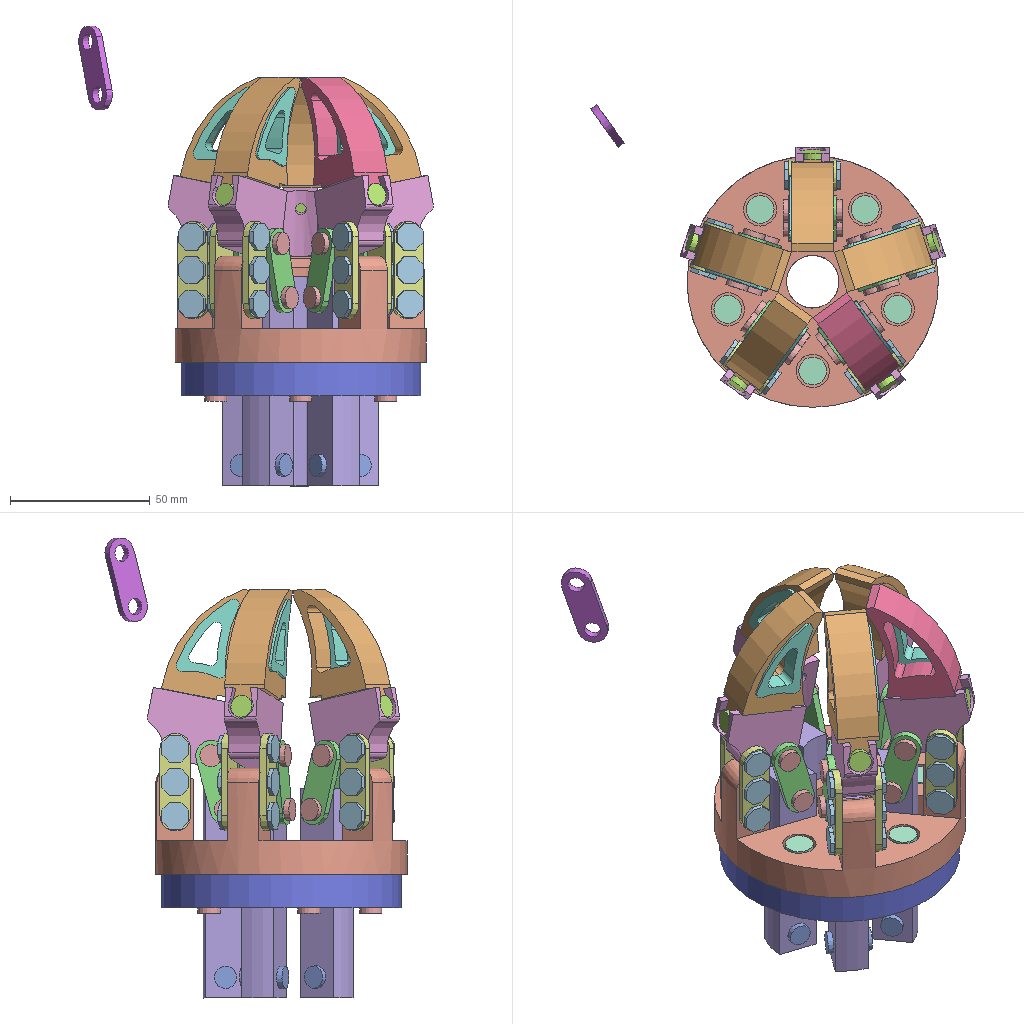Assembly | NX | 14 different items | 123 placed | box 127 x 108 x 165 mm
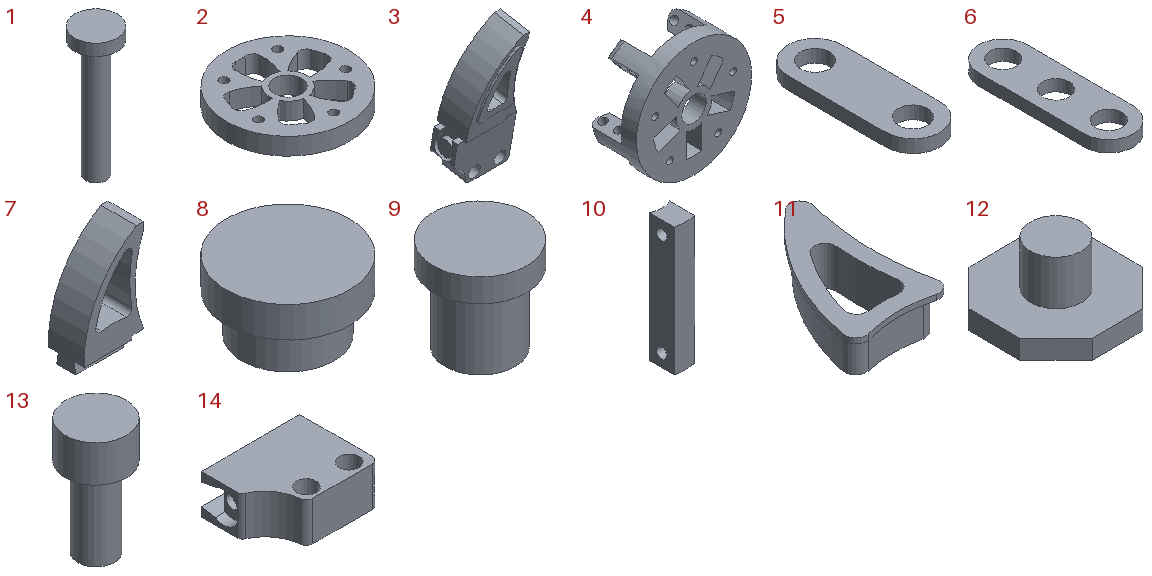Parts list (item | quantity | parent item | size | volume | features):
1 | x5 | in 3 | 8 x 8 x 24.4 mm | 389.557 mm3 | features DATUM_CSYS 2, EXTRUDE 2, SKETCH 1
2 | x1 | - | 86 x 86 x 12 mm | 44699 mm3 | features DATUM_CSYS 4, EXTRUDE 4, SKETCH 3
3 | x5 | - | - | 14028 mm3 | features DATUM_CSYS 17, EXTRUDE 15, SKETCH 13, CPROJ 4, BLEND 2
4 | x1 | - | 90 x 38 x 90 mm | 71655 mm3 | features DATUM_CSYS 9, SKETCH 8, EXTRUDE 7, CBORE_HOLE 5, CPROJ 1, HOLE PACKAGE 1, SWP104 1
5 | x11 | - | 11 x 31 x 2.6 mm | 672.06 mm3 | features DATUM_CSYS 2, EXTRUDE 1, SKETCH 1
6 | x10 | - | 11 x 35 x 2.6 mm | 712.946 mm3 | features DATUM_CSYS 2, EXTRUDE 1, SKETCH 1
7 | x5 | in 3 | - | 6914 mm3 | features DATUM_CSYS 4, EXTRUDE 3, SKETCH 3, CPROJ 2
8 | x25 | - | 8 x 8 x 4.5 mm | 171.217 mm3 | features CYLINDER 2, DATUM_CSYS 1
9 | x10 | - | 8 x 8 x 8 mm | 270.177 mm3 | features CYLINDER 2, DATUM_CSYS 1
10 | x5 | - | 12 x 15.351 x 75 mm | 12124 mm3 | features DATUM_CSYS 3, EXTRUDE 2, SKETCH 2
11 | x5 | in 3 | 18.409 x 28.891 x 7.4 mm | 1102 mm3 | features DATUM_CSYS 4, EXTRUDE 3, SKETCH 3, BLEND 1, CPROJ 1
12 | x30 | - | 9.657 x 9.657 x 5 mm | 159.865 mm3 | features DATUM_CSYS 2, EXTRUDE 2, SKETCH 1
13 | x5 | - | 10 x 10 x 19 mm | 838.805 mm3 | features DATUM_CSYS 2, EXTRUDE 2, SKETCH 1
14 | x5 | in 3 | 30 x 24 x 12 mm | 5622 mm3 | features DATUM_CSYS 7, EXTRUDE 7, SKETCH 6, BLEND 1, CPROJ 1
Mates (type | each side: item.copy, entity, surface, feature):
In the top assembly
Fix | assembly component | 6 times
Bond | 12.1 component | assembly component | 34 times
Bond | assembly component | 20 times
LinearPattern | assembly axis | assembly csys | assembly csys | assembly csys | 2 times
Bond | 6.1 component | assembly component | 10 times
CircularPattern | assembly axis | assembly csys | assembly csys | assembly csys | assembly csys | assembly csys | 16 times
Bond | 5.1 component | assembly component | 15 times
LinearPattern | assembly axis | assembly csys | assembly csys | 2 times
Bond | 10.1 component | assembly component | 6 times
Bond | 3.1 component | assembly component | 6 times
Fix | 4.1 component
Fix | 2.1 component
Fix | 12.1 component | 30 times
Parallel | 10.1 face plane Extrude(2) | 4.1 face plane Revolve(2)
Touch | 10.1 face cylinder Extrude(2) | 4.1 face cylinder Extrude(6)
Fix | 6.1 component | 2 times
Concentric | 5.1 edge | 14.1 edge | 2 times
Concentric | 5.1 edge | 10.1 edge | 2 times
Concentric | 14.1 edge | 6.1 edge
Concentric | 9.1 edge | 10.1 edge | 2 times
Concentric | 8.1 edge | 5.1 edge | 4 times
Concentric | 8.1 edge | 2.1 edge
In subassembly 3
Fix | 14.1 component | 2 times
Fix | 7.1 component
Touch | 7.1 | 11.1
Concentric | 1.1 | 14.1